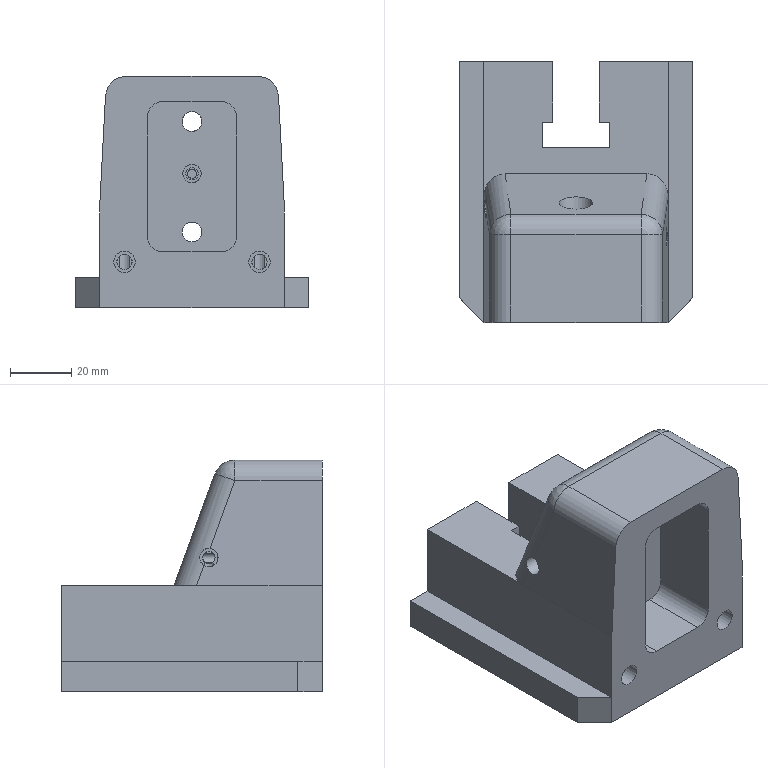Part | NX | features solid 2 | 1 solid | 99 faces | box 76 x 85 x 75.5 mm | volume 224951 mm3 | plane 54 | cylinder 41 | sphere 2 | cone 2 | commonest cylinder face diameters 5 x14 4 x5 14 x5 7 x4 10 x4 6 x3